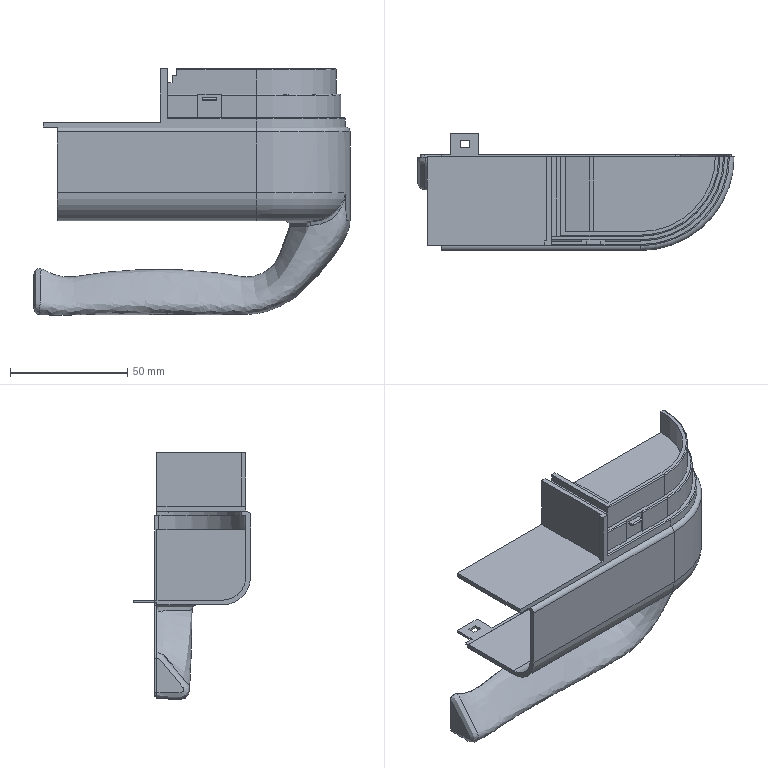Part | SolidWorks | features ICE 9, Fillet 6, BossThin 3, CombineBodies 1, CompositeCurve 1, SewRefSurface 1, Shell 1, Stock 1, SurfCut 1, Sweep 1 | 1 solid | 132 faces | box 135 x 50.019 x 105.415 mm | volume 48449 mm3 | plane 87 | cylinder 23 | spline 16 | torus 6 | commonest cylinder face diameters 1 x6 4 x2 20 x2 24 x2 68 x2 72 x2